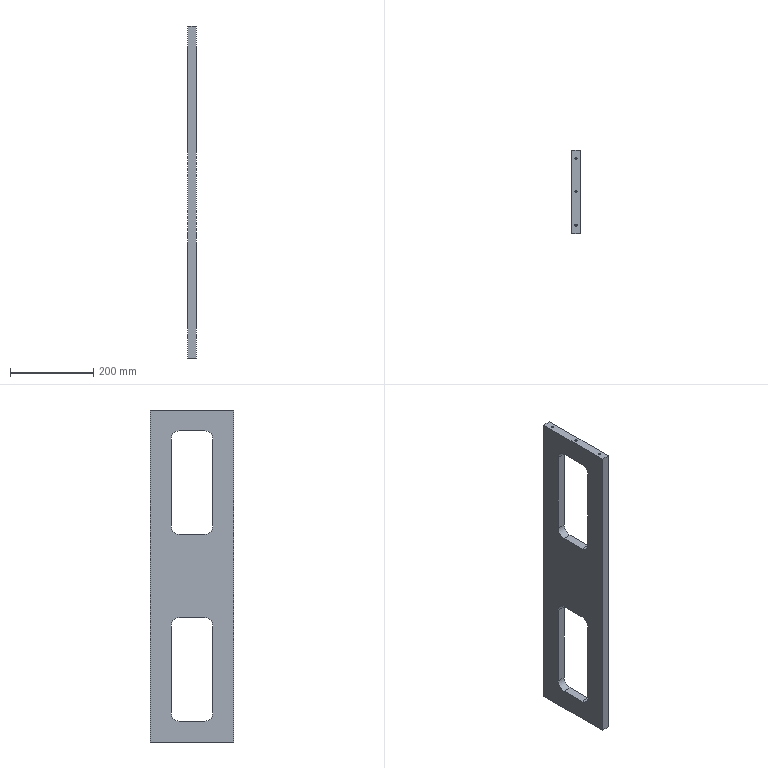Part | STEP file | 0244_211_Plate | 1 solid | 46 faces | box 20 x 200 x 796 mm | volume 2203908 mm3 | cylinder 20 | plane 14 | cone 12 | commonest cylinder face diameters 5 x12 40 x8